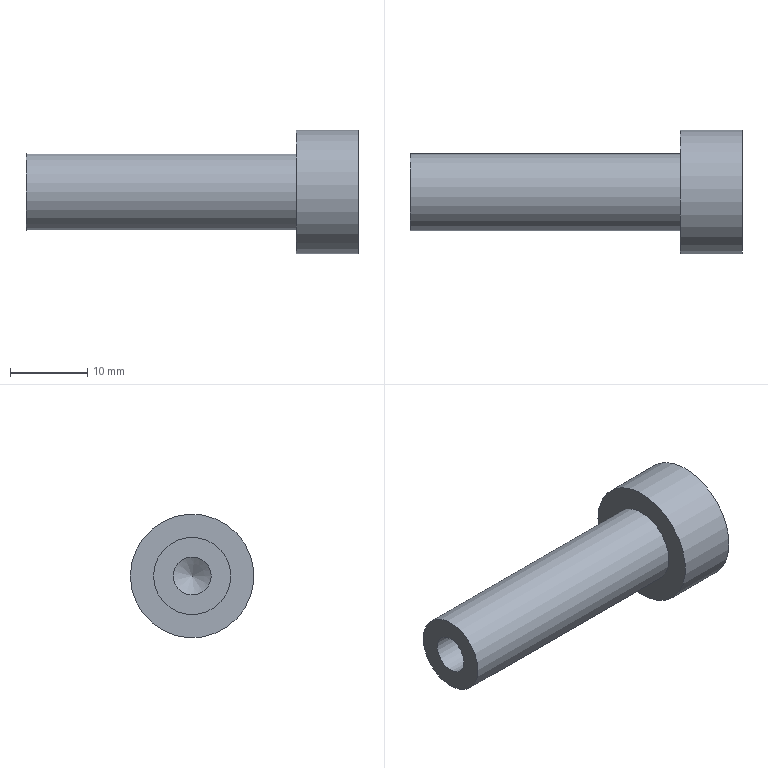Part | NX | features 5003_315_PBTN10-LC35 2 | 1 solid | 20 faces | box 43 x 16 x 16 mm | volume 3884 mm3 | plane 15 | cylinder 3 | cone 2 | commonest cylinder face diameters 4.917 x1 10 x1 16 x1
STEP:
#1=CARTESIAN_POINT('',(-197.475,-526.,-143.536));
#2=VERTEX_POINT('',#1);
#3=CARTESIAN_POINT('',(-197.475,-529.,-145.268));
#4=VERTEX_POINT('',#3);
#5=CARTESIAN_POINT('',(-197.475,-526.,-143.536));
#6=DIRECTION('',(0.,-0.866,-0.5));
#7=VECTOR('',#6,1000.);
#8=LINE('',#5,#7);
#9=EDGE_CURVE('',#2,#4,#8,.T.);
#10=ORIENTED_EDGE('',*,*,#9,.F.);
#11=CARTESIAN_POINT('',(-197.475,-523.,-145.268));
#12=VERTEX_POINT('',#11);
#13=CARTESIAN_POINT('',(-197.475,-523.,-145.268));
#14=DIRECTION('',(0.,-0.866,0.5));
#15=VECTOR('',#14,1000.);
#16=LINE('',#13,#15);
#17=EDGE_CURVE('',#12,#2,#16,.T.);
#18=ORIENTED_EDGE('',*,*,#17,.F.);
#19=CARTESIAN_POINT('',(-197.475,-523.,-148.732));
#20=VERTEX_POINT('',#19);
#21=CARTESIAN_POINT('',(-197.475,-523.,-148.732));
#22=DIRECTION('',(0.,0.,1.));
#23=VECTOR('',#22,1000.);
#24=LINE('',#21,#23);
#25=EDGE_CURVE('',#20,#12,#24,.T.);
#26=ORIENTED_EDGE('',*,*,#25,.F.);
#27=CARTESIAN_POINT('',(-197.475,-526.,-150.464));
#28=VERTEX_POINT('',#27);
#29=CARTESIAN_POINT('',(-197.475,-526.,-150.464));
#30=DIRECTION('',(0.,0.866,0.5));
#31=VECTOR('',#30,1000.);
#32=LINE('',#29,#31);
#33=EDGE_CURVE('',#28,#20,#32,.T.);
#34=ORIENTED_EDGE('',*,*,#33,.F.);
#35=CARTESIAN_POINT('',(-197.475,-529.,-148.732));
#36=VERTEX_POINT('',#35);
#37=CARTESIAN_POINT('',(-197.475,-529.,-148.732));
#38=DIRECTION('',(0.,0.866,-0.5));
#39=VECTOR('',#38,1000.);
#40=LINE('',#37,#39);
#41=EDGE_CURVE('',#36,#28,#40,.T.);
#42=ORIENTED_EDGE('',*,*,#41,.F.);
#43=CARTESIAN_POINT('',(-197.475,-529.,-145.268));
#44=DIRECTION('',(0.,0.,-1.));
#45=VECTOR('',#44,1000.);
#46=LINE('',#43,#45);
#47=EDGE_CURVE('',#4,#36,#46,.T.);
#48=ORIENTED_EDGE('',*,*,#47,.F.);
#49=EDGE_LOOP('',(#10,#18,#26,#34,#42,#48));
#50=FACE_BOUND('',#49,.T.);
#51=CARTESIAN_POINT('',(-197.475,-518.,-147.));
#52=VERTEX_POINT('',#51);
#53=CARTESIAN_POINT('',(-197.475,-526.,-147.));
#54=DIRECTION('',(1.,0.,0.));
#55=DIRECTION('',(0.,1.,0.));
#56=AXIS2_PLACEMENT_3D('',#53,#54,#55);
#57=CIRCLE('',#56,8.);
#58=EDGE_CURVE('',#52,#52,#57,.T.);
#59=ORIENTED_EDGE('',*,*,#58,.T.);
#60=EDGE_LOOP('',(#59));
#61=FACE_BOUND('',#60,.T.);
#62=CARTESIAN_POINT('',(-197.475,-526.,-147.));
#63=DIRECTION('',(-1.,0.,0.));
#64=DIRECTION('',(0.,-1.,0.));
#65=AXIS2_PLACEMENT_3D('',#62,#63,#64);
#66=PLANE('',#65);
#67=ADVANCED_FACE('',(#50,#61),#66,.F.);
#68=ORIENTED_EDGE('',*,*,#58,.F.);
#69=EDGE_LOOP('',(#68));
#70=FACE_BOUND('',#69,.T.);
#71=CARTESIAN_POINT('',(-205.475,-518.,-147.));
#72=VERTEX_POINT('',#71);
#73=CARTESIAN_POINT('',(-205.475,-526.,-147.));
#74=DIRECTION('',(1.,0.,0.));
#75=DIRECTION('',(0.,1.,0.));
#76=AXIS2_PLACEMENT_3D('',#73,#74,#75);
#77=CIRCLE('',#76,8.);
#78=EDGE_CURVE('',#72,#72,#77,.T.);
#79=ORIENTED_EDGE('',*,*,#78,.T.);
#80=EDGE_LOOP('',(#79));
#81=FACE_BOUND('',#80,.T.);
#82=CARTESIAN_POINT('',(-197.475,-526.,-147.));
#83=DIRECTION('',(1.,0.,0.));
#84=DIRECTION('',(0.,1.,0.));
#85=AXIS2_PLACEMENT_3D('',#82,#83,#84);
#86=CYLINDRICAL_SURFACE('',#85,8.);
#87=ADVANCED_FACE('',(#70,#81),#86,.T.);
#88=ORIENTED_EDGE('',*,*,#78,.F.);
#89=EDGE_LOOP('',(#88));
#90=FACE_BOUND('',#89,.T.);
#91=CARTESIAN_POINT('',(-205.475,-521.,-147.));
#92=VERTEX_POINT('',#91);
#93=CARTESIAN_POINT('',(-205.475,-526.,-147.));
#94=DIRECTION('',(1.,0.,0.));
#95=DIRECTION('',(0.,1.,0.));
#96=AXIS2_PLACEMENT_3D('',#93,#94,#95);
#97=CIRCLE('',#96,5.);
#98=EDGE_CURVE('',#92,#92,#97,.T.);
#99=ORIENTED_EDGE('',*,*,#98,.T.);
#100=EDGE_LOOP('',(#99));
#101=FACE_BOUND('',#100,.T.);
#102=CARTESIAN_POINT('',(-205.475,-531.,-147.));
#103=DIRECTION('',(1.,0.,0.));
#104=DIRECTION('',(0.,1.,0.));
#105=AXIS2_PLACEMENT_3D('',#102,#103,#104);
#106=PLANE('',#105);
#107=ADVANCED_FACE('',(#90,#101),#106,.F.);
#108=ORIENTED_EDGE('',*,*,#98,.F.);
#109=EDGE_LOOP('',(#108));
#110=FACE_BOUND('',#109,.T.);
#111=CARTESIAN_POINT('',(-240.475,-521.,-147.));
#112=VERTEX_POINT('',#111);
#113=CARTESIAN_POINT('',(-240.475,-526.,-147.));
#114=DIRECTION('',(1.,0.,0.));
#115=DIRECTION('',(0.,1.,0.));
#116=AXIS2_PLACEMENT_3D('',#113,#114,#115);
#117=CIRCLE('',#116,5.);
#118=EDGE_CURVE('',#112,#112,#117,.T.);
#119=ORIENTED_EDGE('',*,*,#118,.T.);
#120=EDGE_LOOP('',(#119));
#121=FACE_BOUND('',#120,.T.);
#122=CARTESIAN_POINT('',(-197.475,-526.,-147.));
#123=DIRECTION('',(1.,0.,0.));
#124=DIRECTION('',(0.,1.,0.));
#125=AXIS2_PLACEMENT_3D('',#122,#123,#124);
#126=CYLINDRICAL_SURFACE('',#125,5.);
#127=ADVANCED_FACE('',(#110,#121),#126,.T.);
#128=CARTESIAN_POINT('',(-240.475,-528.458,-147.));
#129=VERTEX_POINT('',#128);
#130=CARTESIAN_POINT('',(-240.475,-526.,-147.));
#131=DIRECTION('',(-1.,0.,0.));
#132=DIRECTION('',(0.,-1.,0.));
#133=AXIS2_PLACEMENT_3D('',#130,#131,#132);
#134=CIRCLE('',#133,2.458);
#135=EDGE_CURVE('',#129,#129,#134,.T.);
#136=ORIENTED_EDGE('',*,*,#135,.F.);
#137=EDGE_LOOP('',(#136));
#138=FACE_BOUND('',#137,.T.);
#139=ORIENTED_EDGE('',*,*,#118,.F.);
#140=EDGE_LOOP('',(#139));
#141=FACE_BOUND('',#140,.T.);
#142=CARTESIAN_POINT('',(-240.475,-531.,-147.));
#143=DIRECTION('',(1.,0.,0.));
#144=DIRECTION('',(0.,1.,0.));
#145=AXIS2_PLACEMENT_3D('',#142,#143,#144);
#146=PLANE('',#145);
#147=ADVANCED_FACE('',(#138,#141),#146,.F.);
#148=CARTESIAN_POINT('',(-221.998,-526.,-147.));
#149=VERTEX_POINT('',#148);
#150=VERTEX_LOOP('',#149);
#151=FACE_BOUND('',#150,.T.);
#152=CARTESIAN_POINT('',(-223.475,-528.458,-147.));
#153=VERTEX_POINT('',#152);
#154=CARTESIAN_POINT('',(-223.475,-526.,-147.));
#155=DIRECTION('',(-1.,0.,0.));
#156=DIRECTION('',(0.,-1.,0.));
#157=AXIS2_PLACEMENT_3D('',#154,#155,#156);
#158=CIRCLE('',#157,2.458);
#159=EDGE_CURVE('',#153,#153,#158,.T.);
#160=ORIENTED_EDGE('',*,*,#159,.T.);
#161=EDGE_LOOP('',(#160));
#162=FACE_BOUND('',#161,.T.);
#163=CARTESIAN_POINT('',(-223.475,-526.,-147.));
#164=DIRECTION('',(-1.,0.,0.));
#165=DIRECTION('',(0.,-1.,0.));
#166=AXIS2_PLACEMENT_3D('',#163,#164,#165);
#167=CONICAL_SURFACE('',#166,2.458,1.03);
#168=ADVANCED_FACE('',(#151,#162),#167,.F.);
#169=ORIENTED_EDGE('',*,*,#159,.F.);
#170=EDGE_LOOP('',(#169));
#171=FACE_BOUND('',#170,.T.);
#172=ORIENTED_EDGE('',*,*,#135,.T.);
#173=EDGE_LOOP('',(#172));
#174=FACE_BOUND('',#173,.T.);
#175=CARTESIAN_POINT('',(-240.475,-526.,-147.));
#176=DIRECTION('',(-1.,0.,0.));
#177=DIRECTION('',(0.,-1.,0.));
#178=AXIS2_PLACEMENT_3D('',#175,#176,#177);
#179=CYLINDRICAL_SURFACE('',#178,2.458);
#180=ADVANCED_FACE('',(#171,#174),#179,.F.);
#181=ORIENTED_EDGE('',*,*,#17,.T.);
#182=CARTESIAN_POINT('',(-201.475,-526.,-143.536));
#183=VERTEX_POINT('',#182);
#184=CARTESIAN_POINT('',(-201.475,-526.,-143.536));
#185=DIRECTION('',(1.,0.,0.));
#186=VECTOR('',#185,1000.);
#187=LINE('',#184,#186);
#188=EDGE_CURVE('',#183,#2,#187,.T.);
#189=ORIENTED_EDGE('',*,*,#188,.F.);
#190=CARTESIAN_POINT('',(-201.475,-523.,-145.268));
#191=VERTEX_POINT('',#190);
#192=CARTESIAN_POINT('',(-201.475,-523.,-145.268));
#193=DIRECTION('',(0.,-0.866,0.5));
#194=VECTOR('',#193,1000.);
#195=LINE('',#192,#194);
#196=EDGE_CURVE('',#191,#183,#195,.T.);
#197=ORIENTED_EDGE('',*,*,#196,.F.);
#198=CARTESIAN_POINT('',(-201.475,-523.,-145.268));
#199=DIRECTION('',(1.,0.,0.));
#200=VECTOR('',#199,1000.);
#201=LINE('',#198,#200);
#202=EDGE_CURVE('',#191,#12,#201,.T.);
#203=ORIENTED_EDGE('',*,*,#202,.T.);
#204=EDGE_LOOP('',(#181,#189,#197,#203));
#205=FACE_BOUND('',#204,.T.);
#206=CARTESIAN_POINT('',(-201.475,-523.,-145.268));
#207=DIRECTION('',(0.,0.5,0.866));
#208=DIRECTION('',(0.,0.866,-0.5));
#209=AXIS2_PLACEMENT_3D('',#206,#207,#208);
#210=PLANE('',#209);
#211=ADVANCED_FACE('',(#205),#210,.F.);
#212=ORIENTED_EDGE('',*,*,#25,.T.);
#213=ORIENTED_EDGE('',*,*,#202,.F.);
#214=CARTESIAN_POINT('',(-201.475,-523.,-148.732));
#215=VERTEX_POINT('',#214);
#216=CARTESIAN_POINT('',(-201.475,-523.,-148.732));
#217=DIRECTION('',(0.,0.,1.));
#218=VECTOR('',#217,1000.);
#219=LINE('',#216,#218);
#220=EDGE_CURVE('',#215,#191,#219,.T.);
#221=ORIENTED_EDGE('',*,*,#220,.F.);
#222=CARTESIAN_POINT('',(-201.475,-523.,-148.732));
#223=DIRECTION('',(1.,0.,0.));
#224=VECTOR('',#223,1000.);
#225=LINE('',#222,#224);
#226=EDGE_CURVE('',#215,#20,#225,.T.);
#227=ORIENTED_EDGE('',*,*,#226,.T.);
#228=EDGE_LOOP('',(#212,#213,#221,#227));
#229=FACE_BOUND('',#228,.T.);
#230=CARTESIAN_POINT('',(-201.475,-523.,-148.732));
#231=DIRECTION('',(0.,1.,0.));
#232=DIRECTION('',(-1.,0.,0.));
#233=AXIS2_PLACEMENT_3D('',#230,#231,#232);
#234=PLANE('',#233);
#235=ADVANCED_FACE('',(#229),#234,.F.);
#236=ORIENTED_EDGE('',*,*,#33,.T.);
#237=ORIENTED_EDGE('',*,*,#226,.F.);
#238=CARTESIAN_POINT('',(-201.475,-526.,-150.464));
#239=VERTEX_POINT('',#238);
#240=CARTESIAN_POINT('',(-201.475,-526.,-150.464));
#241=DIRECTION('',(0.,0.866,0.5));
#242=VECTOR('',#241,1000.);
#243=LINE('',#240,#242);
#244=EDGE_CURVE('',#239,#215,#243,.T.);
#245=ORIENTED_EDGE('',*,*,#244,.F.);
#246=CARTESIAN_POINT('',(-201.475,-526.,-150.464));
#247=DIRECTION('',(1.,0.,0.));
#248=VECTOR('',#247,1000.);
#249=LINE('',#246,#248);
#250=EDGE_CURVE('',#239,#28,#249,.T.);
#251=ORIENTED_EDGE('',*,*,#250,.T.);
#252=EDGE_LOOP('',(#236,#237,#245,#251));
#253=FACE_BOUND('',#252,.T.);
#254=CARTESIAN_POINT('',(-201.475,-526.,-150.464));
#255=DIRECTION('',(0.,0.5,-0.866));
#256=DIRECTION('',(0.,-0.866,-0.5));
#257=AXIS2_PLACEMENT_3D('',#254,#255,#256);
#258=PLANE('',#257);
#259=ADVANCED_FACE('',(#253),#258,.F.);
#260=ORIENTED_EDGE('',*,*,#41,.T.);
#261=ORIENTED_EDGE('',*,*,#250,.F.);
#262=CARTESIAN_POINT('',(-201.475,-529.,-148.732));
#263=VERTEX_POINT('',#262);
#264=CARTESIAN_POINT('',(-201.475,-529.,-148.732));
#265=DIRECTION('',(0.,0.866,-0.5));
#266=VECTOR('',#265,1000.);
#267=LINE('',#264,#266);
#268=EDGE_CURVE('',#263,#239,#267,.T.);
#269=ORIENTED_EDGE('',*,*,#268,.F.);
#270=CARTESIAN_POINT('',(-201.475,-529.,-148.732));
#271=DIRECTION('',(1.,0.,0.));
#272=VECTOR('',#271,1000.);
#273=LINE('',#270,#272);
#274=EDGE_CURVE('',#263,#36,#273,.T.);
#275=ORIENTED_EDGE('',*,*,#274,.T.);
#276=EDGE_LOOP('',(#260,#261,#269,#275));
#277=FACE_BOUND('',#276,.T.);
#278=CARTESIAN_POINT('',(-201.475,-529.,-148.732));
#279=DIRECTION('',(0.,-0.5,-0.866));
#280=DIRECTION('',(0.,-0.866,0.5));
#281=AXIS2_PLACEMENT_3D('',#278,#279,#280);
#282=PLANE('',#281);
#283=ADVANCED_FACE('',(#277),#282,.F.);
#284=ORIENTED_EDGE('',*,*,#47,.T.);
#285=ORIENTED_EDGE('',*,*,#274,.F.);
#286=CARTESIAN_POINT('',(-201.475,-529.,-145.268));
#287=VERTEX_POINT('',#286);
#288=CARTESIAN_POINT('',(-201.475,-529.,-145.268));
#289=DIRECTION('',(0.,0.,-1.));
#290=VECTOR('',#289,1000.);
#291=LINE('',#288,#290);
#292=EDGE_CURVE('',#287,#263,#291,.T.);
#293=ORIENTED_EDGE('',*,*,#292,.F.);
#294=CARTESIAN_POINT('',(-201.475,-529.,-145.268));
#295=DIRECTION('',(1.,0.,0.));
#296=VECTOR('',#295,1000.);
#297=LINE('',#294,#296);
#298=EDGE_CURVE('',#287,#4,#297,.T.);
#299=ORIENTED_EDGE('',*,*,#298,.T.);
#300=EDGE_LOOP('',(#284,#285,#293,#299));
#301=FACE_BOUND('',#300,.T.);
#302=CARTESIAN_POINT('',(-201.475,-529.,-145.268));
#303=DIRECTION('',(0.,-1.,0.));
#304=DIRECTION('',(1.,0.,0.));
#305=AXIS2_PLACEMENT_3D('',#302,#303,#304);
#306=PLANE('',#305);
#307=ADVANCED_FACE('',(#301),#306,.F.);
#308=ORIENTED_EDGE('',*,*,#9,.T.);
#309=ORIENTED_EDGE('',*,*,#298,.F.);
#310=CARTESIAN_POINT('',(-201.475,-526.,-143.536));
#311=DIRECTION('',(0.,-0.866,-0.5));
#312=VECTOR('',#311,1000.);
#313=LINE('',#310,#312);
#314=EDGE_CURVE('',#183,#287,#313,.T.);
#315=ORIENTED_EDGE('',*,*,#314,.F.);
#316=ORIENTED_EDGE('',*,*,#188,.T.);
#317=EDGE_LOOP('',(#308,#309,#315,#316));
#318=FACE_BOUND('',#317,.T.);
#319=CARTESIAN_POINT('',(-201.475,-526.,-143.536));
#320=DIRECTION('',(0.,-0.5,0.866));
#321=DIRECTION('',(0.,0.866,0.5));
#322=AXIS2_PLACEMENT_3D('',#319,#320,#321);
#323=PLANE('',#322);
#324=ADVANCED_FACE('',(#318),#323,.F.);
#325=ORIENTED_EDGE('',*,*,#196,.T.);
#326=CARTESIAN_POINT('',(-201.475,-526.,-147.));
#327=DIRECTION('',(1.,0.,0.));
#328=DIRECTION('',(0.,1.,0.));
#329=AXIS2_PLACEMENT_3D('',#326,#327,#328);
#330=CIRCLE('',#329,3.464);
#331=EDGE_CURVE('',#191,#183,#330,.T.);
#332=ORIENTED_EDGE('',*,*,#331,.F.);
#333=EDGE_LOOP('',(#325,#332));
#334=FACE_BOUND('',#333,.T.);
#335=CARTESIAN_POINT('',(-201.475,-526.,-143.536));
#336=DIRECTION('',(-1.,0.,0.));
#337=DIRECTION('',(0.,-1.,0.));
#338=AXIS2_PLACEMENT_3D('',#335,#336,#337);
#339=PLANE('',#338);
#340=ADVANCED_FACE('',(#334),#339,.T.);
#341=ORIENTED_EDGE('',*,*,#314,.T.);
#342=CARTESIAN_POINT('',(-201.475,-526.,-147.));
#343=DIRECTION('',(1.,0.,0.));
#344=DIRECTION('',(0.,1.,0.));
#345=AXIS2_PLACEMENT_3D('',#342,#343,#344);
#346=CIRCLE('',#345,3.464);
#347=EDGE_CURVE('',#183,#287,#346,.T.);
#348=ORIENTED_EDGE('',*,*,#347,.F.);
#349=EDGE_LOOP('',(#341,#348));
#350=FACE_BOUND('',#349,.T.);
#351=CARTESIAN_POINT('',(-201.475,-526.,-143.536));
#352=DIRECTION('',(-1.,0.,0.));
#353=DIRECTION('',(0.,-1.,0.));
#354=AXIS2_PLACEMENT_3D('',#351,#352,#353);
#355=PLANE('',#354);
#356=ADVANCED_FACE('',(#350),#355,.T.);
#357=ORIENTED_EDGE('',*,*,#292,.T.);
#358=CARTESIAN_POINT('',(-201.475,-526.,-147.));
#359=DIRECTION('',(1.,0.,0.));
#360=DIRECTION('',(0.,1.,0.));
#361=AXIS2_PLACEMENT_3D('',#358,#359,#360);
#362=CIRCLE('',#361,3.464);
#363=EDGE_CURVE('',#287,#263,#362,.T.);
#364=ORIENTED_EDGE('',*,*,#363,.F.);
#365=EDGE_LOOP('',(#357,#364));
#366=FACE_BOUND('',#365,.T.);
#367=CARTESIAN_POINT('',(-201.475,-526.,-143.536));
#368=DIRECTION('',(-1.,0.,0.));
#369=DIRECTION('',(0.,-1.,0.));
#370=AXIS2_PLACEMENT_3D('',#367,#368,#369);
#371=PLANE('',#370);
#372=ADVANCED_FACE('',(#366),#371,.T.);
#373=ORIENTED_EDGE('',*,*,#268,.T.);
#374=CARTESIAN_POINT('',(-201.475,-526.,-147.));
#375=DIRECTION('',(1.,0.,0.));
#376=DIRECTION('',(0.,1.,0.));
#377=AXIS2_PLACEMENT_3D('',#374,#375,#376);
#378=CIRCLE('',#377,3.464);
#379=EDGE_CURVE('',#263,#239,#378,.T.);
#380=ORIENTED_EDGE('',*,*,#379,.F.);
#381=EDGE_LOOP('',(#373,#380));
#382=FACE_BOUND('',#381,.T.);
#383=CARTESIAN_POINT('',(-201.475,-526.,-143.536));
#384=DIRECTION('',(-1.,0.,0.));
#385=DIRECTION('',(0.,-1.,0.));
#386=AXIS2_PLACEMENT_3D('',#383,#384,#385);
#387=PLANE('',#386);
#388=ADVANCED_FACE('',(#382),#387,.T.);
#389=ORIENTED_EDGE('',*,*,#244,.T.);
#390=CARTESIAN_POINT('',(-201.475,-526.,-147.));
#391=DIRECTION('',(1.,0.,0.));
#392=DIRECTION('',(0.,1.,0.));
#393=AXIS2_PLACEMENT_3D('',#390,#391,#392);
#394=CIRCLE('',#393,3.464);
#395=EDGE_CURVE('',#239,#215,#394,.T.);
#396=ORIENTED_EDGE('',*,*,#395,.F.);
#397=EDGE_LOOP('',(#389,#396));
#398=FACE_BOUND('',#397,.T.);
#399=CARTESIAN_POINT('',(-201.475,-526.,-143.536));
#400=DIRECTION('',(-1.,0.,0.));
#401=DIRECTION('',(0.,-1.,0.));
#402=AXIS2_PLACEMENT_3D('',#399,#400,#401);
#403=PLANE('',#402);
#404=ADVANCED_FACE('',(#398),#403,.T.);
#405=ORIENTED_EDGE('',*,*,#220,.T.);
#406=CARTESIAN_POINT('',(-201.475,-526.,-147.));
#407=DIRECTION('',(1.,0.,0.));
#408=DIRECTION('',(0.,1.,0.));
#409=AXIS2_PLACEMENT_3D('',#406,#407,#408);
#410=CIRCLE('',#409,3.464);
#411=EDGE_CURVE('',#215,#191,#410,.T.);
#412=ORIENTED_EDGE('',*,*,#411,.F.);
#413=EDGE_LOOP('',(#405,#412));
#414=FACE_BOUND('',#413,.T.);
#415=CARTESIAN_POINT('',(-201.475,-526.,-143.536));
#416=DIRECTION('',(-1.,0.,0.));
#417=DIRECTION('',(0.,-1.,0.));
#418=AXIS2_PLACEMENT_3D('',#415,#416,#417);
#419=PLANE('',#418);
#420=ADVANCED_FACE('',(#414),#419,.T.);
#421=ORIENTED_EDGE('',*,*,#331,.T.);
#422=ORIENTED_EDGE('',*,*,#347,.T.);
#423=ORIENTED_EDGE('',*,*,#363,.T.);
#424=ORIENTED_EDGE('',*,*,#379,.T.);
#425=ORIENTED_EDGE('',*,*,#395,.T.);
#426=ORIENTED_EDGE('',*,*,#411,.T.);
#427=EDGE_LOOP('',(#421,#422,#423,#424,#425,#426));
#428=FACE_BOUND('',#427,.T.);
#429=CARTESIAN_POINT('',(-202.775,-526.,-147.));
#430=VERTEX_POINT('',#429);
#431=VERTEX_LOOP('',#430);
#432=FACE_BOUND('',#431,.T.);
#433=CARTESIAN_POINT('',(-202.775,-526.,-147.));
#434=DIRECTION('',(1.,0.,0.));
#435=DIRECTION('',(0.,1.,0.));
#436=AXIS2_PLACEMENT_3D('',#433,#434,#435);
#437=CONICAL_SURFACE('',#436,0.,1.212);
#438=ADVANCED_FACE('',(#428,#432),#437,.F.);
#439=CLOSED_SHELL('',(#67,#87,#107,#127,#147,#168,#180,#211,#235,#259,#283,#307,#324,#340,#356,#372,#388,#404,#420,#438));
#440=MANIFOLD_SOLID_BREP('',#439);
#441=(LENGTH_UNIT()NAMED_UNIT(*)SI_UNIT(.MILLI.,.METRE.));
#442=UNCERTAINTY_MEASURE_WITH_UNIT(LENGTH_MEASURE(0.00001),#441,'','');
#443=(NAMED_UNIT(*)PLANE_ANGLE_UNIT()SI_UNIT($,.RADIAN.));
#444=(NAMED_UNIT(*)SI_UNIT($,.STERADIAN.)SOLID_ANGLE_UNIT());
#445=(GEOMETRIC_REPRESENTATION_CONTEXT(3)GLOBAL_UNCERTAINTY_ASSIGNED_CONTEXT((#442))GLOBAL_UNIT_ASSIGNED_CONTEXT((#441,#443,#444))REPRESENTATION_CONTEXT('',''));
#446=ADVANCED_BREP_SHAPE_REPRESENTATION('',(#440),#445);